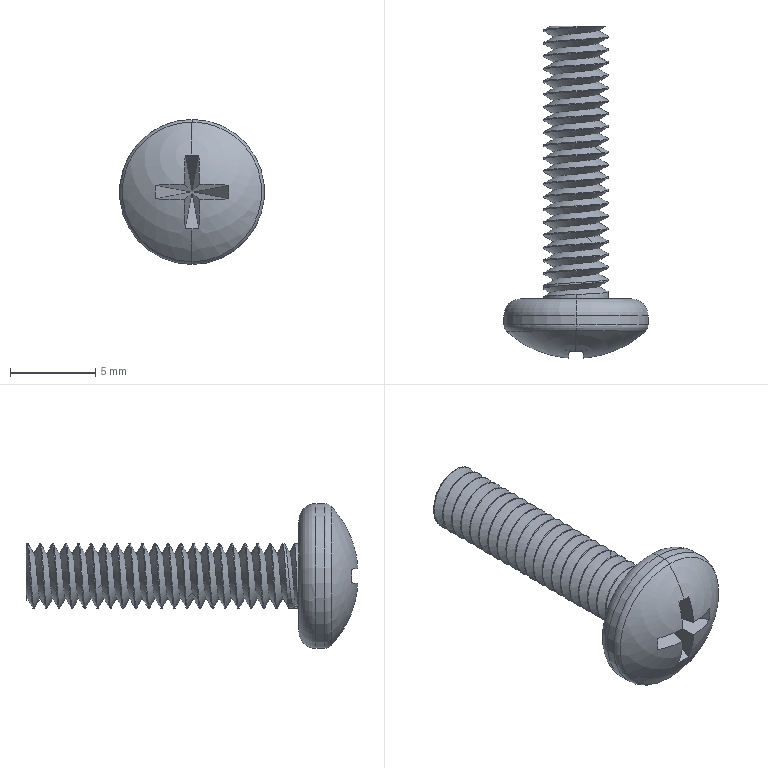Part | STEP file | _X2_751F4E45_X0_MS731-1_X2_8_10 | 1 solid | 82 faces | box 8.5 x 19.466 x 8.5 mm | volume 271.985 mm3 | cylinder 44 | plane 16 | spline 15 | torus 4 | sphere 2 | other 1 | commonest cylinder face diameters 3.8 x42 8.5 x2